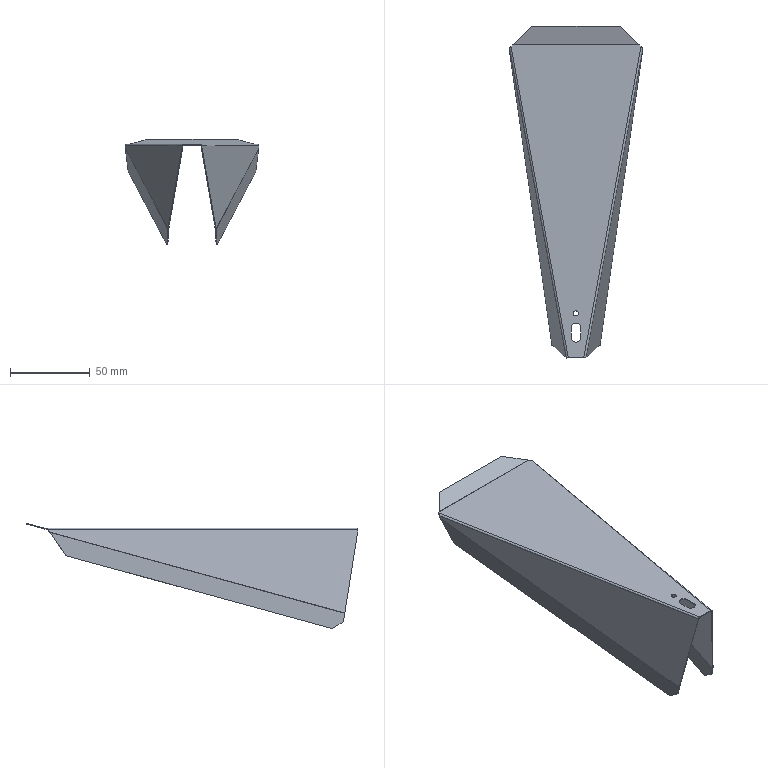Part | SolidWorks | features BaseBody 1 | 1 solid | 56 faces | box 83.843 x 208.675 x 66.218 mm | volume 12643 mm3 | plane 32 | cylinder 14 | spline 10 | commonest cylinder face diameters 1.5 x5 2.5 x5 3.2 x2 6 x2